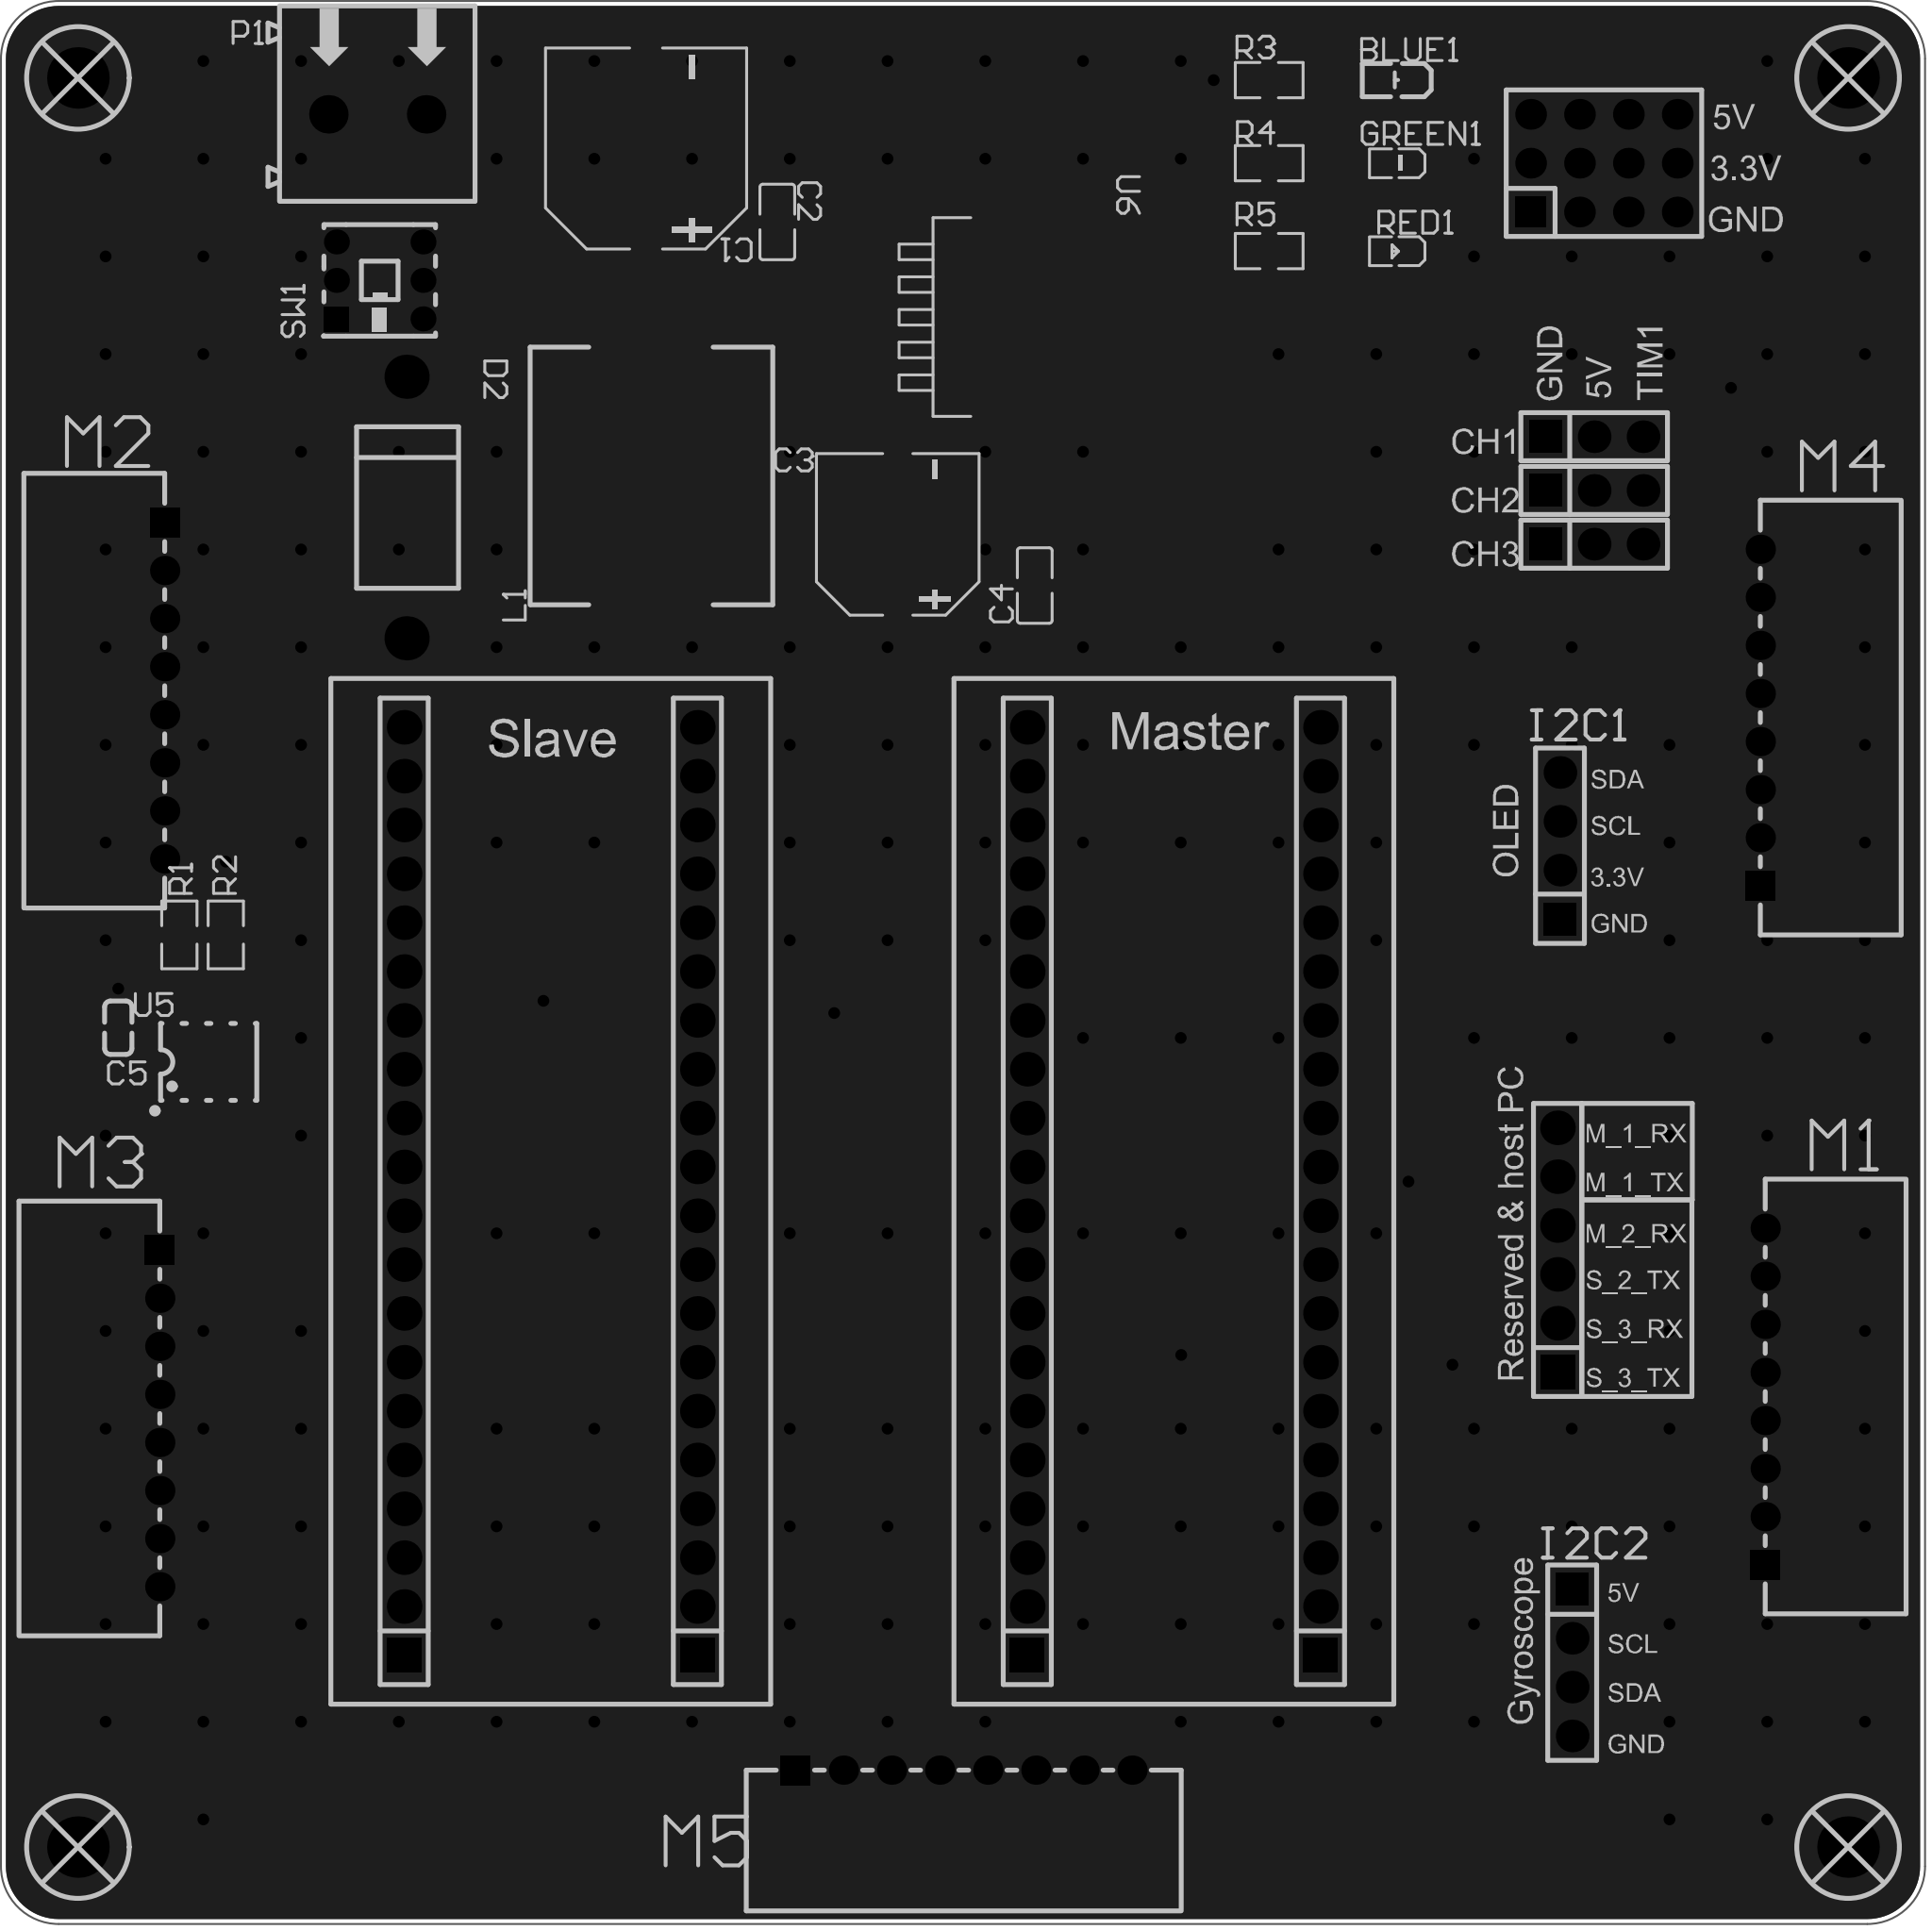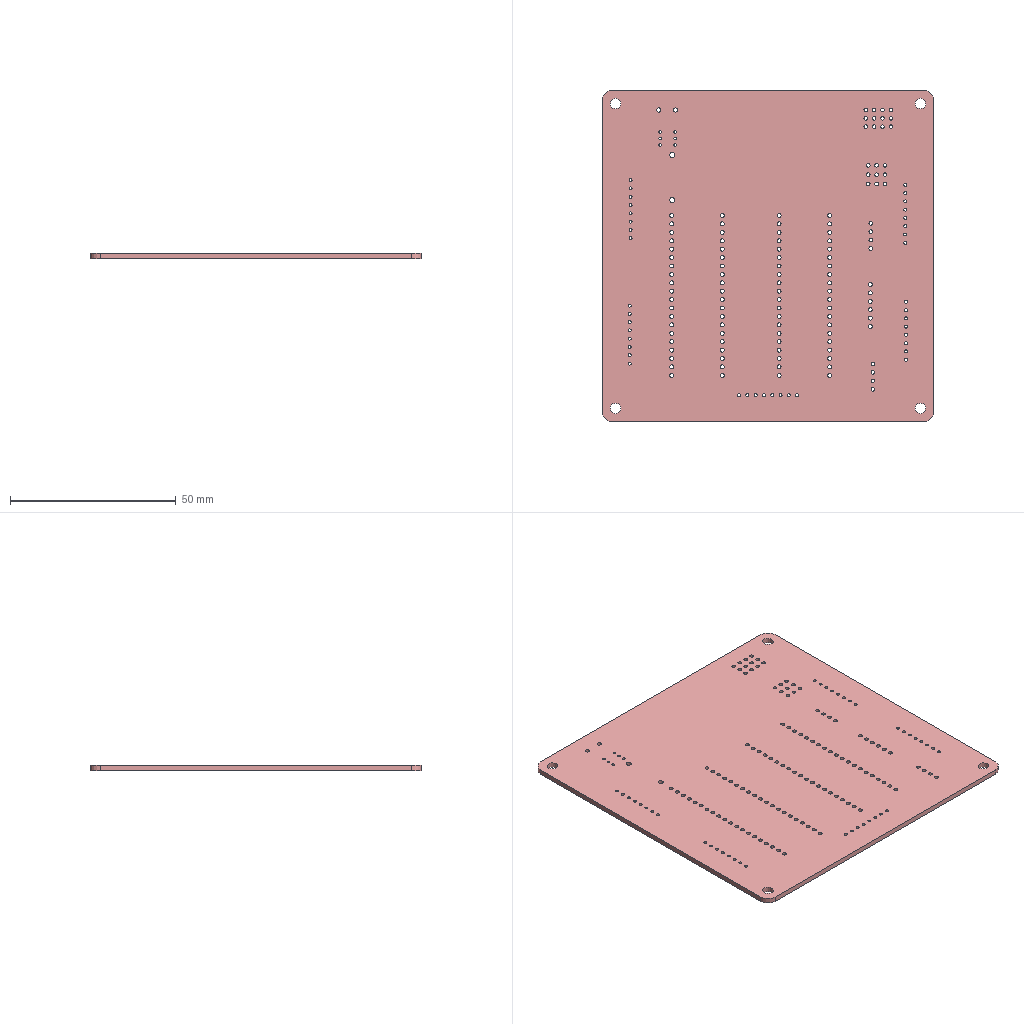Circuit board layout | Altium Designer | box 100 x 100 x 1.6 mm
Layer stack:
# Altium Designer layer stack of  (unit mm; dielectric type: 0 none, 1 core, 2 prepreg, 3 surface material)
index,name,kind,layer,copper_thickness_mm,dielectric_type,dielectric_thickness_mm,dielectric_material,dielectric_constant
0,Top Paste Mask Layer,other,,,,,,
1,Top Silkscreen Layer,other,,,,,,
2,Top Solder Mask Layer,dielectric,,,3,0,,0
3,Top Layer,copper,Top Layer,0.035,,,,
4,Dielectric1,dielectric,,,3,0.2104,7628 RC49% 8.6mil,0
5,Inner1,copper,Inner1,0.0152,,,,
6,Dielectric2,dielectric,,,3,1.065,1.1mm H/HOZ Copper,0
7,Inner2,copper,Inner2,0.0152,,,,
8,Dielectric3,dielectric,,,3,0.2104,7628 RC49% 8.6mil,0
9,Bottom Layer,copper,Bottom Layer,0.035,,,,
10,Bottom Solder Mask Layer,dielectric,,,3,0,,0
11,Bottom Silkscreen Layer,other,,,,,,
12,Bottom Paste Mask Layer,other,,,,,,
# drill layer pairs: low layer,high layer
drill_pair,Top Layer,Bottom Layer
Part placement:
Designator,Comment,Layer,Footprint,Center-X(mm),Center-Y(mm),Rotation
BLUE1,SZYY0603B,TopLayer,LED0603-R-RD_BLUE,148.717,172.085,180
C1,220uF,TopLayer,CAP-SMD_BD10.0-L10.3-W10.3-FD,109.728,168.529,90
C2,100nF,TopLayer,C0805,116.549,164.71,270
C3,680uF,TopLayer,CAP-SMD_BD8.0-L8.3-W8.3-FD,122.809,148.463,90
C4,100nF,TopLayer,C0805,129.928,145.803,270
D2,1N5824,TopLayer,DO-27_BD5.3-L8.4-P12.40-D1.3-RD,97.282,149.86,270
GREEN1,XL-1608PGC-06,TopLayer,LED0603-RD_GREEN,148.717,167.767,180
H1,PZ254V-11-03P,TopLayer,HDR-TH_3P-P2.54-V-M,159.004,153.543,0
H2,PZ254V-11-03P,TopLayer,HDR-TH_3P-P2.54-V-M,159.004,150.749,0
H3,PZ254V-11-03P,TopLayer,HDR-TH_3P-P2.54-V-M,159.004,147.955,0
L1,33uH,TopLayer,IND-SMD_L13.45-W12.6,109.982,151.511,90
P1,WJ500V-5.08-2P,TopLayer,CONN-TH_2P-P5.00_WJ500V-5.08-2P,95.758,170.307,0
R3,3K,TopLayer,R0805,142.113,172.085,180
R4,1K,TopLayer,R0805,142.113,167.767,180
R5,550Ω,TopLayer,R0805,142.113,163.195,180
RED1,XL-1608SURC-06,TopLayer,LED0603-RD_RED,148.717,163.195,180
SW1,5.8 WSPT,TopLayer,SW-TH_6P-L5.8-W5.8-P2.00-LS4.5-TL_K8-5851E-L1,95.885,161.671,90
U6,LM2596S-ADJ,TopLayer,TO-263-5_L10.2-W8.6-P1.70-LS14.4-BR,125.984,159.766,180
U2,ZX-PM2.54-1-20PY,TopLayer,HDR-TH_20P-P2.54-V-F,144.78,114.3,90
U4,ZX-PM2.54-1-20PY,TopLayer,HDR-TH_20P-P2.54-V-F,112.395,114.3,90
U1,ZX-PM2.54-1-20PY,TopLayer,HDR-TH_20P-P2.54-V-F,129.54,114.3,90
U3,ZX-PM2.54-1-20PY,TopLayer,HDR-TH_20P-P2.54-V-F,97.155,114.3,90
M1,ZX-XH2.54-8PWZ,TopLayer,CONN-TH_8P-P2.50_ZX-XH2.54-8PWZ,167.894,103.632,90
M2,ZX-XH2.54-8PWZ,TopLayer,CONN-TH_8P-P2.50_ZX-XH2.54-8PWZ,84.709,140.335,270
M4,ZX-XH2.54-8PWZ,TopLayer,CONN-TH_8P-P2.50_ZX-XH2.54-8PWZ,167.64,138.938,90
M5,ZX-XH2.54-8PWZ,TopLayer,CONN-TH_8P-P2.50_ZX-XH2.54-8PWZ,126.238,84.201,0
M3,ZX-XH2.54-8PWZ,TopLayer,CONN-TH_8P-P2.50_ZX-XH2.54-8PWZ,84.455,102.489,270
H4,PZ254V-11-04P,TopLayer,HDR-TH_4P-P2.54-V-M,157.861,89.789,270
H5,2.54-1x6P straight pin,TopLayer,HDR-TH_6P-P2.54-V-M-1,157.099,111.252,90
H6,PZ254V-11-04P,TopLayer,HDR-TH_4P-P2.54-V-M,157.226,132.272,90
U12,HX PZ2.54-3x4P ZZ,TopLayer,HDR-TH_12P-P2.54-V-M-R3-C4-S2.54,159.512,167.767,0
SCREW1,,TopLayer,M3螺丝,80.2,172.2,0
SCREW2,,TopLayer,M3螺丝,172.2,172.2,0
SCREW3,,TopLayer,M3螺丝,80.2,80.2,0
SCREW4,,TopLayer,M3螺丝,172.2,80.2,0
U5,MAX3485ESA-MS,TopLayer,SO-8_L4.9-W3.9-P1.27-LS5.9-BL,86.995,121.031,0
C5,100nF,TopLayer,C0603,82.296,122.809,270
R1,4.7kΩ,TopLayer,R0805,85.471,127.635,90
R2,4.7kΩ,TopLayer,R0805,87.884,127.635,90
Pad and via stacks:
# Altium Designer via and pad stacks of  (unit mm). Each distinct definition once, with the count of objects using it.
# via: kind,start_layer,end_layer,hole_mm,diameter_mm,mode(0 simple;1 top-mid-bottom;2 full stack),diameter_per_layer,count,example_net
# pad: kind,layer,hole_mm,hole_type(0 round;1 square;2 slot),plating,top_size,top_shape(1 round;2 rect;3 octagon;9 rounded rect),mid_size,bottom_size,mode,footprint,size_per_layer,count,example
pad,Top Layer,0,0,plated,0.8x0.8,2,0.8x0.8,0.8x0.8,0,LED0603-R-RD_BLUE,,2,BLUE1.2
pad,Top Layer,0,0,plated,4.5x1.65,2,4.5x1.65,4.5x1.65,0,CAP-SMD_BD10.0-L10.3-W10.3-FD,,2,C1.1
pad,Top Layer,0,0,plated,1.41x1.35,2,1.41x1.35,1.41x1.35,0,C0805,,4,C2.2
pad,Top Layer,0,0,plated,4.2x1.4,2,4.2x1.4,4.2x1.4,0,CAP-SMD_BD8.0-L8.3-W8.3-FD,,2,C3.1
pad,Top Layer,0,0,plated,0.8x0.8,2,0.8x0.8,0.8x0.8,0,LED0603-RD_GREEN,,2,GREEN1.1
pad,Top Layer,0,0,plated,3x6,2,3x6,3x6,0,IND-SMD_L13.45-W12.6,,2,L1.2
pad,Top Layer,0,0,plated,1.133x1.377,2,1.133x1.377,1.133x1.377,0,R0805,,10,R3.2
pad,Top Layer,0,0,plated,0.8x0.8,2,0.8x0.8,0.8x0.8,0,LED0603-RD_RED,,2,RED1.1
pad,Top Layer,0,0,plated,3.5x1.02,2,3.5x1.02,3.5x1.02,0,TO-263-5_L10.2-W8.6-P1.70-LS14.4-BR,,5,U6.1
pad,Top Layer,0,0,plated,8.705x10.587,2,8.705x10.587,8.705x10.587,0,TO-263-5_L10.2-W8.6-P1.70-LS14.4-BR,,1,U6.6
pad,Top Layer,0,0,plated,0.574x1.888,1,0.574x1.888,0.574x1.888,0,SO-8_L4.9-W3.9-P1.27-LS5.9-BL,,8,U5.1
pad,Top Layer,0,0,plated,0.8x0.9,2,0.8x0.9,0.8x0.9,0,C0603,,2,C5.2
pad,Multi-Layer,1.5,0,plated,2.3x2.3,1,2.3x2.3,2.3x2.3,0,DO-27_BD5.3-L8.4-P12.40-D1.3-RD,,2,D2.2
pad,Multi-Layer,1.1,0,plated,1.7x1.7,2,1.7x1.7,1.7x1.7,0,HDR-TH_3P-P2.54-V-M,,3,H1.1
pad,Multi-Layer,1.1,0,plated,1.7x1.7,1,1.7x1.7,1.7x1.7,0,HDR-TH_3P-P2.54-V-M,,6,H1.2
pad,Multi-Layer,1.3,0,plated,2x2,1,2x2,2x2,0,CONN-TH_2P-P5.00_WJ500V-5.08-2P,,2,P1.2
pad,Multi-Layer,0.8,0,plated,1.3x1.3,2,1.3x1.3,1.3x1.3,0,SW-TH_6P-L5.8-W5.8-P2.00-LS4.5-TL_K8-5851E-L1,,1,SW1.1
pad,Multi-Layer,0.8,0,plated,1.3x1.3,1,1.3x1.3,1.3x1.3,0,SW-TH_6P-L5.8-W5.8-P2.00-LS4.5-TL_K8-5851E-L1,,5,SW1.2
pad,Multi-Layer,1.2,0,plated,1.8x1.8,2,1.8x1.8,1.8x1.8,0,HDR-TH_20P-P2.54-V-F,,4,U2.1
pad,Multi-Layer,1.2,0,plated,1.8x1.8,1,1.8x1.8,1.8x1.8,0,HDR-TH_20P-P2.54-V-F,,76,U2.2
pad,Multi-Layer,0.9144,0,plated,1.524x1.524,2,1.524x1.524,1.524x1.524,0,CONN-TH_8P-P2.50_ZX-XH2.54-8PWZ,,5,M1.1
pad,Multi-Layer,0.9144,0,plated,1.524x1.524,1,1.524x1.524,1.524x1.524,0,CONN-TH_8P-P2.50_ZX-XH2.54-8PWZ,,35,M1.2
pad,Multi-Layer,1.1,0,plated,1.7x1.7,2,1.7x1.7,1.7x1.7,0,HDR-TH_4P-P2.54-V-M,,2,H4.1
pad,Multi-Layer,1.1,0,plated,1.7x1.7,1,1.7x1.7,1.7x1.7,0,HDR-TH_4P-P2.54-V-M,,6,H4.2
pad,Multi-Layer,1.2,0,plated,1.8x1.8,1,1.8x1.8,1.8x1.8,0,HDR-TH_6P-P2.54-V-M-1,,5,H5.6
pad,Multi-Layer,1.2,0,plated,1.8x1.8,2,1.8x1.8,1.8x1.8,0,HDR-TH_6P-P2.54-V-M-1,,1,H5.1
pad,Multi-Layer,1.1,0,plated,1.6x1.6,2,1.6x1.6,1.6x1.6,0,HDR-TH_12P-P2.54-V-M-R3-C4-S2.54,,1,U12.1
pad,Multi-Layer,1.1,0,plated,1.6x1.6,1,1.6x1.6,1.6x1.6,0,HDR-TH_12P-P2.54-V-M-R3-C4-S2.54,,11,U12.2
pad,Multi-Layer,3.2,0,plated,3.2x3.2,1,3.2x3.2,3.2x3.2,0,M3\u00C2\u00DD\u00CB\u00BF,,4,SCREW1.1
via,Top Layer,Bottom Layer,0.3048,0.61,0,,230,3.3V
Copper pours:
name,layer,net,type(0 solid;1 hatched;2 none)
Top Layer-GND,Top Layer,GND,0
Inner2-GND,Inner2,GND,0
Inner1-GND,Inner1,GND,0
Bottom Layer-GND,Bottom Layer,GND,0
Design rules, without the lines most boards share:
# Altium Designer design rules of  (exported by Altium Designer, unit mm)
# columns: name | kind | enabled | priority | scope1 | scope2 | descriptor | typed fields (field=value)
20mil | 2 | enabled | 2 | (InNet('5V') OR InNet('3.3V')) | All | Width Constraint (Min=5mil) (Max=100mil) (Preferred=20mil) ((InNet('5V') OR InNet('3.3V'))) |
30mil | 2 | enabled | 3 | (InNet('12.6V')) | All | Width Constraint (Min=5mil) (Max=100mil) (Preferred=30mil) ((InNet('12.6V'))) |
copperThickness1oz_2 | 2 | enabled | 4 | All | All | Width Constraint (Min=5mil) (Max=100mil) (Preferred=10mil) (All) |